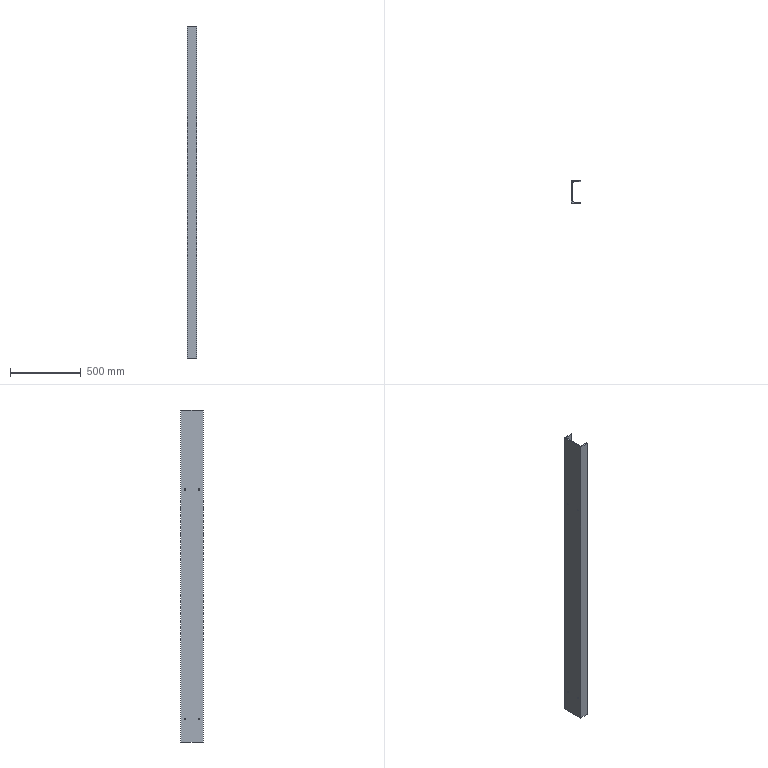Part | SolidWorks | features Extrusion 1, HoleWzd 1 | 1 solid | 18 faces | box 65 x 160 x 2340 mm | volume 4766991 mm3 | plane 10 | cylinder 8 | commonest cylinder face diameters 8.5 x8
STEP:
#1=CARTESIAN_POINT('',(8.5,30.,-1014.25));
#2=VERTEX_POINT('',#1);
#3=CARTESIAN_POINT('',(8.5,30.,-1005.75));
#4=VERTEX_POINT('',#3);
#5=CARTESIAN_POINT('',(8.5,30.,-1010.));
#6=DIRECTION('',(-1.,0.,0.));
#7=DIRECTION('',(0.,0.,1.));
#8=AXIS2_PLACEMENT_3D('',#5,#6,#7);
#9=CIRCLE('',#8,4.25);
#10=EDGE_CURVE('',#2,#4,#9,.T.);
#11=ORIENTED_EDGE('',*,*,#10,.F.);
#12=CARTESIAN_POINT('',(0.,30.,-1014.25));
#13=VERTEX_POINT('',#12);
#14=CARTESIAN_POINT('',(0.,30.,-1014.25));
#15=DIRECTION('',(-1.,0.,0.));
#16=VECTOR('',#15,1000.);
#17=LINE('',#14,#16);
#18=EDGE_CURVE('',#2,#13,#17,.T.);
#19=ORIENTED_EDGE('',*,*,#18,.T.);
#20=CARTESIAN_POINT('',(0.,30.,-1005.75));
#21=VERTEX_POINT('',#20);
#22=CARTESIAN_POINT('',(0.,30.,-1010.));
#23=DIRECTION('',(-1.,0.,0.));
#24=DIRECTION('',(0.,0.,1.));
#25=AXIS2_PLACEMENT_3D('',#22,#23,#24);
#26=CIRCLE('',#25,4.25);
#27=EDGE_CURVE('',#13,#21,#26,.T.);
#28=ORIENTED_EDGE('',*,*,#27,.T.);
#29=CARTESIAN_POINT('',(0.,30.,-1005.75));
#30=DIRECTION('',(-1.,0.,0.));
#31=VECTOR('',#30,1000.);
#32=LINE('',#29,#31);
#33=EDGE_CURVE('',#4,#21,#32,.T.);
#34=ORIENTED_EDGE('',*,*,#33,.F.);
#35=EDGE_LOOP('',(#11,#19,#28,#34));
#36=FACE_OUTER_BOUND('',#35,.T.);
#37=CARTESIAN_POINT('',(0.,30.,-1010.));
#38=DIRECTION('',(-1.,0.,0.));
#39=DIRECTION('',(0.,0.,1.));
#40=AXIS2_PLACEMENT_3D('',#37,#38,#39);
#41=CYLINDRICAL_SURFACE('',#40,4.25);
#42=ADVANCED_FACE('',(#36),#41,.F.);
#43=CARTESIAN_POINT('',(8.5,30.,605.75));
#44=VERTEX_POINT('',#43);
#45=CARTESIAN_POINT('',(8.5,30.,614.25));
#46=VERTEX_POINT('',#45);
#47=CARTESIAN_POINT('',(8.5,30.,610.));
#48=DIRECTION('',(-1.,0.,0.));
#49=DIRECTION('',(0.,0.,1.));
#50=AXIS2_PLACEMENT_3D('',#47,#48,#49);
#51=CIRCLE('',#50,4.25);
#52=EDGE_CURVE('',#44,#46,#51,.T.);
#53=ORIENTED_EDGE('',*,*,#52,.F.);
#54=CARTESIAN_POINT('',(0.,30.,605.75));
#55=VERTEX_POINT('',#54);
#56=CARTESIAN_POINT('',(0.,30.,605.75));
#57=DIRECTION('',(-1.,0.,0.));
#58=VECTOR('',#57,1000.);
#59=LINE('',#56,#58);
#60=EDGE_CURVE('',#44,#55,#59,.T.);
#61=ORIENTED_EDGE('',*,*,#60,.T.);
#62=CARTESIAN_POINT('',(0.,30.,614.25));
#63=VERTEX_POINT('',#62);
#64=CARTESIAN_POINT('',(0.,30.,610.));
#65=DIRECTION('',(-1.,0.,0.));
#66=DIRECTION('',(0.,0.,1.));
#67=AXIS2_PLACEMENT_3D('',#64,#65,#66);
#68=CIRCLE('',#67,4.25);
#69=EDGE_CURVE('',#55,#63,#68,.T.);
#70=ORIENTED_EDGE('',*,*,#69,.T.);
#71=CARTESIAN_POINT('',(0.,30.,614.25));
#72=DIRECTION('',(-1.,0.,0.));
#73=VECTOR('',#72,1000.);
#74=LINE('',#71,#73);
#75=EDGE_CURVE('',#46,#63,#74,.T.);
#76=ORIENTED_EDGE('',*,*,#75,.F.);
#77=EDGE_LOOP('',(#53,#61,#70,#76));
#78=FACE_OUTER_BOUND('',#77,.T.);
#79=CARTESIAN_POINT('',(0.,30.,610.));
#80=DIRECTION('',(-1.,0.,0.));
#81=DIRECTION('',(0.,0.,1.));
#82=AXIS2_PLACEMENT_3D('',#79,#80,#81);
#83=CYLINDRICAL_SURFACE('',#82,4.25);
#84=ADVANCED_FACE('',(#78),#83,.F.);
#85=CARTESIAN_POINT('',(8.5,130.,605.75));
#86=VERTEX_POINT('',#85);
#87=CARTESIAN_POINT('',(8.5,130.,614.25));
#88=VERTEX_POINT('',#87);
#89=CARTESIAN_POINT('',(8.5,130.,610.));
#90=DIRECTION('',(-1.,0.,0.));
#91=DIRECTION('',(0.,0.,1.));
#92=AXIS2_PLACEMENT_3D('',#89,#90,#91);
#93=CIRCLE('',#92,4.25);
#94=EDGE_CURVE('',#86,#88,#93,.T.);
#95=ORIENTED_EDGE('',*,*,#94,.F.);
#96=CARTESIAN_POINT('',(0.,130.,605.75));
#97=VERTEX_POINT('',#96);
#98=CARTESIAN_POINT('',(0.,130.,605.75));
#99=DIRECTION('',(-1.,0.,0.));
#100=VECTOR('',#99,1000.);
#101=LINE('',#98,#100);
#102=EDGE_CURVE('',#86,#97,#101,.T.);
#103=ORIENTED_EDGE('',*,*,#102,.T.);
#104=CARTESIAN_POINT('',(0.,130.,614.25));
#105=VERTEX_POINT('',#104);
#106=CARTESIAN_POINT('',(0.,130.,610.));
#107=DIRECTION('',(-1.,0.,0.));
#108=DIRECTION('',(0.,0.,1.));
#109=AXIS2_PLACEMENT_3D('',#106,#107,#108);
#110=CIRCLE('',#109,4.25);
#111=EDGE_CURVE('',#97,#105,#110,.T.);
#112=ORIENTED_EDGE('',*,*,#111,.T.);
#113=CARTESIAN_POINT('',(0.,130.,614.25));
#114=DIRECTION('',(-1.,0.,0.));
#115=VECTOR('',#114,1000.);
#116=LINE('',#113,#115);
#117=EDGE_CURVE('',#88,#105,#116,.T.);
#118=ORIENTED_EDGE('',*,*,#117,.F.);
#119=EDGE_LOOP('',(#95,#103,#112,#118));
#120=FACE_OUTER_BOUND('',#119,.T.);
#121=CARTESIAN_POINT('',(0.,130.,610.));
#122=DIRECTION('',(-1.,0.,0.));
#123=DIRECTION('',(0.,0.,1.));
#124=AXIS2_PLACEMENT_3D('',#121,#122,#123);
#125=CYLINDRICAL_SURFACE('',#124,4.25);
#126=ADVANCED_FACE('',(#120),#125,.F.);
#127=CARTESIAN_POINT('',(8.5,130.,-1014.25));
#128=VERTEX_POINT('',#127);
#129=CARTESIAN_POINT('',(8.5,130.,-1005.75));
#130=VERTEX_POINT('',#129);
#131=CARTESIAN_POINT('',(8.5,130.,-1010.));
#132=DIRECTION('',(-1.,0.,0.));
#133=DIRECTION('',(0.,0.,1.));
#134=AXIS2_PLACEMENT_3D('',#131,#132,#133);
#135=CIRCLE('',#134,4.25);
#136=EDGE_CURVE('',#128,#130,#135,.T.);
#137=ORIENTED_EDGE('',*,*,#136,.F.);
#138=CARTESIAN_POINT('',(0.,130.,-1014.25));
#139=VERTEX_POINT('',#138);
#140=CARTESIAN_POINT('',(0.,130.,-1014.25));
#141=DIRECTION('',(-1.,0.,0.));
#142=VECTOR('',#141,1000.);
#143=LINE('',#140,#142);
#144=EDGE_CURVE('',#128,#139,#143,.T.);
#145=ORIENTED_EDGE('',*,*,#144,.T.);
#146=CARTESIAN_POINT('',(0.,130.,-1005.75));
#147=VERTEX_POINT('',#146);
#148=CARTESIAN_POINT('',(0.,130.,-1010.));
#149=DIRECTION('',(-1.,0.,0.));
#150=DIRECTION('',(0.,0.,1.));
#151=AXIS2_PLACEMENT_3D('',#148,#149,#150);
#152=CIRCLE('',#151,4.25);
#153=EDGE_CURVE('',#139,#147,#152,.T.);
#154=ORIENTED_EDGE('',*,*,#153,.T.);
#155=CARTESIAN_POINT('',(0.,130.,-1005.75));
#156=DIRECTION('',(-1.,0.,0.));
#157=VECTOR('',#156,1000.);
#158=LINE('',#155,#157);
#159=EDGE_CURVE('',#130,#147,#158,.T.);
#160=ORIENTED_EDGE('',*,*,#159,.F.);
#161=EDGE_LOOP('',(#137,#145,#154,#160));
#162=FACE_OUTER_BOUND('',#161,.T.);
#163=CARTESIAN_POINT('',(0.,130.,-1010.));
#164=DIRECTION('',(-1.,0.,0.));
#165=DIRECTION('',(0.,0.,1.));
#166=AXIS2_PLACEMENT_3D('',#163,#164,#165);
#167=CYLINDRICAL_SURFACE('',#166,4.25);
#168=ADVANCED_FACE('',(#162),#167,.F.);
#169=CARTESIAN_POINT('',(0.,30.,-1010.));
#170=DIRECTION('',(-1.,0.,0.));
#171=DIRECTION('',(0.,0.,1.));
#172=AXIS2_PLACEMENT_3D('',#169,#170,#171);
#173=CIRCLE('',#172,4.25);
#174=EDGE_CURVE('',#21,#13,#173,.T.);
#175=ORIENTED_EDGE('',*,*,#174,.F.);
#176=ORIENTED_EDGE('',*,*,#27,.F.);
#177=EDGE_LOOP('',(#175,#176));
#178=FACE_BOUND('',#177,.T.);
#179=CARTESIAN_POINT('',(0.,30.,610.));
#180=DIRECTION('',(-1.,0.,0.));
#181=DIRECTION('',(0.,0.,1.));
#182=AXIS2_PLACEMENT_3D('',#179,#180,#181);
#183=CIRCLE('',#182,4.25);
#184=EDGE_CURVE('',#63,#55,#183,.T.);
#185=ORIENTED_EDGE('',*,*,#184,.F.);
#186=ORIENTED_EDGE('',*,*,#69,.F.);
#187=EDGE_LOOP('',(#185,#186));
#188=FACE_BOUND('',#187,.T.);
#189=CARTESIAN_POINT('',(0.,130.,610.));
#190=DIRECTION('',(-1.,0.,0.));
#191=DIRECTION('',(0.,0.,1.));
#192=AXIS2_PLACEMENT_3D('',#189,#190,#191);
#193=CIRCLE('',#192,4.25);
#194=EDGE_CURVE('',#105,#97,#193,.T.);
#195=ORIENTED_EDGE('',*,*,#194,.F.);
#196=ORIENTED_EDGE('',*,*,#111,.F.);
#197=EDGE_LOOP('',(#195,#196));
#198=FACE_BOUND('',#197,.T.);
#199=CARTESIAN_POINT('',(0.,130.,-1010.));
#200=DIRECTION('',(-1.,0.,0.));
#201=DIRECTION('',(0.,0.,1.));
#202=AXIS2_PLACEMENT_3D('',#199,#200,#201);
#203=CIRCLE('',#202,4.25);
#204=EDGE_CURVE('',#147,#139,#203,.T.);
#205=ORIENTED_EDGE('',*,*,#204,.F.);
#206=ORIENTED_EDGE('',*,*,#153,.F.);
#207=EDGE_LOOP('',(#205,#206));
#208=FACE_BOUND('',#207,.T.);
#209=CARTESIAN_POINT('',(0.,160.,-1170.));
#210=VERTEX_POINT('',#209);
#211=CARTESIAN_POINT('',(0.,0.,-1170.));
#212=VERTEX_POINT('',#211);
#213=CARTESIAN_POINT('',(0.,0.,-1170.));
#214=DIRECTION('',(0.,-1.,0.));
#215=VECTOR('',#214,1000.);
#216=LINE('',#213,#215);
#217=EDGE_CURVE('',#210,#212,#216,.T.);
#218=ORIENTED_EDGE('',*,*,#217,.T.);
#219=CARTESIAN_POINT('',(0.,0.,1170.));
#220=VERTEX_POINT('',#219);
#221=CARTESIAN_POINT('',(0.,0.,1170.));
#222=DIRECTION('',(0.,0.,-1.));
#223=VECTOR('',#222,1000.);
#224=LINE('',#221,#223);
#225=EDGE_CURVE('',#220,#212,#224,.T.);
#226=ORIENTED_EDGE('',*,*,#225,.F.);
#227=CARTESIAN_POINT('',(0.,160.,1170.));
#228=VERTEX_POINT('',#227);
#229=CARTESIAN_POINT('',(0.,0.,1170.));
#230=DIRECTION('',(0.,-1.,0.));
#231=VECTOR('',#230,1000.);
#232=LINE('',#229,#231);
#233=EDGE_CURVE('',#228,#220,#232,.T.);
#234=ORIENTED_EDGE('',*,*,#233,.F.);
#235=CARTESIAN_POINT('',(0.,160.,1170.));
#236=DIRECTION('',(0.,0.,-1.));
#237=VECTOR('',#236,1000.);
#238=LINE('',#235,#237);
#239=EDGE_CURVE('',#228,#210,#238,.T.);
#240=ORIENTED_EDGE('',*,*,#239,.T.);
#241=EDGE_LOOP('',(#218,#226,#234,#240));
#242=FACE_OUTER_BOUND('',#241,.T.);
#243=CARTESIAN_POINT('',(0.,0.,1170.));
#244=DIRECTION('',(1.,0.,0.));
#245=DIRECTION('',(0.,0.,-1.));
#246=AXIS2_PLACEMENT_3D('',#243,#244,#245);
#247=PLANE('',#246);
#248=ADVANCED_FACE('',(#178,#188,#198,#208,#242),#247,.F.);
#249=CARTESIAN_POINT('',(65.,0.,-1170.));
#250=VERTEX_POINT('',#249);
#251=CARTESIAN_POINT('',(0.,0.,-1170.));
#252=DIRECTION('',(1.,0.,0.));
#253=VECTOR('',#252,1000.);
#254=LINE('',#251,#253);
#255=EDGE_CURVE('',#212,#250,#254,.T.);
#256=ORIENTED_EDGE('',*,*,#255,.T.);
#257=CARTESIAN_POINT('',(65.,0.,1170.));
#258=VERTEX_POINT('',#257);
#259=CARTESIAN_POINT('',(65.,0.,1170.));
#260=DIRECTION('',(0.,0.,-1.));
#261=VECTOR('',#260,1000.);
#262=LINE('',#259,#261);
#263=EDGE_CURVE('',#258,#250,#262,.T.);
#264=ORIENTED_EDGE('',*,*,#263,.F.);
#265=CARTESIAN_POINT('',(0.,0.,1170.));
#266=DIRECTION('',(1.,0.,0.));
#267=VECTOR('',#266,1000.);
#268=LINE('',#265,#267);
#269=EDGE_CURVE('',#220,#258,#268,.T.);
#270=ORIENTED_EDGE('',*,*,#269,.F.);
#271=ORIENTED_EDGE('',*,*,#225,.T.);
#272=EDGE_LOOP('',(#256,#264,#270,#271));
#273=FACE_OUTER_BOUND('',#272,.T.);
#274=CARTESIAN_POINT('',(0.,0.,1170.));
#275=DIRECTION('',(0.,1.,0.));
#276=DIRECTION('',(0.,0.,1.));
#277=AXIS2_PLACEMENT_3D('',#274,#275,#276);
#278=PLANE('',#277);
#279=ADVANCED_FACE('',(#273),#278,.F.);
#280=CARTESIAN_POINT('',(65.,4.,-1170.));
#281=VERTEX_POINT('',#280);
#282=CARTESIAN_POINT('',(65.,0.,-1170.));
#283=DIRECTION('',(0.,1.,0.));
#284=VECTOR('',#283,1000.);
#285=LINE('',#282,#284);
#286=EDGE_CURVE('',#250,#281,#285,.T.);
#287=ORIENTED_EDGE('',*,*,#286,.T.);
#288=CARTESIAN_POINT('',(65.,4.,1170.));
#289=VERTEX_POINT('',#288);
#290=CARTESIAN_POINT('',(65.,4.,1170.));
#291=DIRECTION('',(0.,0.,-1.));
#292=VECTOR('',#291,1000.);
#293=LINE('',#290,#292);
#294=EDGE_CURVE('',#289,#281,#293,.T.);
#295=ORIENTED_EDGE('',*,*,#294,.F.);
#296=CARTESIAN_POINT('',(65.,0.,1170.));
#297=DIRECTION('',(0.,1.,0.));
#298=VECTOR('',#297,1000.);
#299=LINE('',#296,#298);
#300=EDGE_CURVE('',#258,#289,#299,.T.);
#301=ORIENTED_EDGE('',*,*,#300,.F.);
#302=ORIENTED_EDGE('',*,*,#263,.T.);
#303=EDGE_LOOP('',(#287,#295,#301,#302));
#304=FACE_OUTER_BOUND('',#303,.T.);
#305=CARTESIAN_POINT('',(65.,0.,1170.));
#306=DIRECTION('',(-1.,0.,0.));
#307=DIRECTION('',(0.,0.,1.));
#308=AXIS2_PLACEMENT_3D('',#305,#306,#307);
#309=PLANE('',#308);
#310=ADVANCED_FACE('',(#304),#309,.F.);
#311=CARTESIAN_POINT('',(8.5,8.,-1170.));
#312=VERTEX_POINT('',#311);
#313=CARTESIAN_POINT('',(65.,4.,-1170.));
#314=DIRECTION('',(-0.9975,0.07062,0.));
#315=VECTOR('',#314,1000.);
#316=LINE('',#313,#315);
#317=EDGE_CURVE('',#281,#312,#316,.T.);
#318=ORIENTED_EDGE('',*,*,#317,.T.);
#319=CARTESIAN_POINT('',(8.5,8.,1170.));
#320=VERTEX_POINT('',#319);
#321=CARTESIAN_POINT('',(8.5,8.,1170.));
#322=DIRECTION('',(0.,0.,-1.));
#323=VECTOR('',#322,1000.);
#324=LINE('',#321,#323);
#325=EDGE_CURVE('',#320,#312,#324,.T.);
#326=ORIENTED_EDGE('',*,*,#325,.F.);
#327=CARTESIAN_POINT('',(65.,4.,1170.));
#328=DIRECTION('',(-0.9975,0.07062,0.));
#329=VECTOR('',#328,1000.);
#330=LINE('',#327,#329);
#331=EDGE_CURVE('',#289,#320,#330,.T.);
#332=ORIENTED_EDGE('',*,*,#331,.F.);
#333=ORIENTED_EDGE('',*,*,#294,.T.);
#334=EDGE_LOOP('',(#318,#326,#332,#333));
#335=FACE_OUTER_BOUND('',#334,.T.);
#336=CARTESIAN_POINT('',(65.,4.,1170.));
#337=DIRECTION('',(-0.07062,-0.9975,0.));
#338=DIRECTION('',(0.9975,-0.07062,0.));
#339=AXIS2_PLACEMENT_3D('',#336,#337,#338);
#340=PLANE('',#339);
#341=ADVANCED_FACE('',(#335),#340,.F.);
#342=CARTESIAN_POINT('',(8.5,30.,-1010.));
#343=DIRECTION('',(-1.,0.,0.));
#344=DIRECTION('',(0.,0.,1.));
#345=AXIS2_PLACEMENT_3D('',#342,#343,#344);
#346=CIRCLE('',#345,4.25);
#347=EDGE_CURVE('',#4,#2,#346,.T.);
#348=ORIENTED_EDGE('',*,*,#347,.T.);
#349=ORIENTED_EDGE('',*,*,#10,.T.);
#350=EDGE_LOOP('',(#348,#349));
#351=FACE_BOUND('',#350,.T.);
#352=CARTESIAN_POINT('',(8.5,30.,610.));
#353=DIRECTION('',(-1.,0.,0.));
#354=DIRECTION('',(0.,0.,1.));
#355=AXIS2_PLACEMENT_3D('',#352,#353,#354);
#356=CIRCLE('',#355,4.25);
#357=EDGE_CURVE('',#46,#44,#356,.T.);
#358=ORIENTED_EDGE('',*,*,#357,.T.);
#359=ORIENTED_EDGE('',*,*,#52,.T.);
#360=EDGE_LOOP('',(#358,#359));
#361=FACE_BOUND('',#360,.T.);
#362=CARTESIAN_POINT('',(8.5,130.,610.));
#363=DIRECTION('',(-1.,0.,0.));
#364=DIRECTION('',(0.,0.,1.));
#365=AXIS2_PLACEMENT_3D('',#362,#363,#364);
#366=CIRCLE('',#365,4.25);
#367=EDGE_CURVE('',#88,#86,#366,.T.);
#368=ORIENTED_EDGE('',*,*,#367,.T.);
#369=ORIENTED_EDGE('',*,*,#94,.T.);
#370=EDGE_LOOP('',(#368,#369));
#371=FACE_BOUND('',#370,.T.);
#372=CARTESIAN_POINT('',(8.5,130.,-1010.));
#373=DIRECTION('',(-1.,0.,0.));
#374=DIRECTION('',(0.,0.,1.));
#375=AXIS2_PLACEMENT_3D('',#372,#373,#374);
#376=CIRCLE('',#375,4.25);
#377=EDGE_CURVE('',#130,#128,#376,.T.);
#378=ORIENTED_EDGE('',*,*,#377,.T.);
#379=ORIENTED_EDGE('',*,*,#136,.T.);
#380=EDGE_LOOP('',(#378,#379));
#381=FACE_BOUND('',#380,.T.);
#382=CARTESIAN_POINT('',(8.5,152.,-1170.));
#383=VERTEX_POINT('',#382);
#384=CARTESIAN_POINT('',(8.5,8.,-1170.));
#385=DIRECTION('',(0.,1.,0.));
#386=VECTOR('',#385,1000.);
#387=LINE('',#384,#386);
#388=EDGE_CURVE('',#312,#383,#387,.T.);
#389=ORIENTED_EDGE('',*,*,#388,.T.);
#390=CARTESIAN_POINT('',(8.5,152.,1170.));
#391=VERTEX_POINT('',#390);
#392=CARTESIAN_POINT('',(8.5,152.,1170.));
#393=DIRECTION('',(0.,0.,-1.));
#394=VECTOR('',#393,1000.);
#395=LINE('',#392,#394);
#396=EDGE_CURVE('',#391,#383,#395,.T.);
#397=ORIENTED_EDGE('',*,*,#396,.F.);
#398=CARTESIAN_POINT('',(8.5,8.,1170.));
#399=DIRECTION('',(0.,1.,0.));
#400=VECTOR('',#399,1000.);
#401=LINE('',#398,#400);
#402=EDGE_CURVE('',#320,#391,#401,.T.);
#403=ORIENTED_EDGE('',*,*,#402,.F.);
#404=ORIENTED_EDGE('',*,*,#325,.T.);
#405=EDGE_LOOP('',(#389,#397,#403,#404));
#406=FACE_OUTER_BOUND('',#405,.T.);
#407=CARTESIAN_POINT('',(8.5,8.,1170.));
#408=DIRECTION('',(-1.,0.,0.));
#409=DIRECTION('',(0.,0.,1.));
#410=AXIS2_PLACEMENT_3D('',#407,#408,#409);
#411=PLANE('',#410);
#412=ADVANCED_FACE('',(#351,#361,#371,#381,#406),#411,.F.);
#413=CARTESIAN_POINT('',(65.,156.,-1170.));
#414=VERTEX_POINT('',#413);
#415=CARTESIAN_POINT('',(65.,156.,-1170.));
#416=DIRECTION('',(0.9975,0.07062,0.));
#417=VECTOR('',#416,1000.);
#418=LINE('',#415,#417);
#419=EDGE_CURVE('',#383,#414,#418,.T.);
#420=ORIENTED_EDGE('',*,*,#419,.T.);
#421=CARTESIAN_POINT('',(65.,156.,1170.));
#422=VERTEX_POINT('',#421);
#423=CARTESIAN_POINT('',(65.,156.,1170.));
#424=DIRECTION('',(0.,0.,-1.));
#425=VECTOR('',#424,1000.);
#426=LINE('',#423,#425);
#427=EDGE_CURVE('',#422,#414,#426,.T.);
#428=ORIENTED_EDGE('',*,*,#427,.F.);
#429=CARTESIAN_POINT('',(65.,156.,1170.));
#430=DIRECTION('',(0.9975,0.07062,0.));
#431=VECTOR('',#430,1000.);
#432=LINE('',#429,#431);
#433=EDGE_CURVE('',#391,#422,#432,.T.);
#434=ORIENTED_EDGE('',*,*,#433,.F.);
#435=ORIENTED_EDGE('',*,*,#396,.T.);
#436=EDGE_LOOP('',(#420,#428,#434,#435));
#437=FACE_OUTER_BOUND('',#436,.T.);
#438=CARTESIAN_POINT('',(65.,156.,1170.));
#439=DIRECTION('',(-0.07062,0.9975,0.));
#440=DIRECTION('',(-0.9975,-0.07062,0.));
#441=AXIS2_PLACEMENT_3D('',#438,#439,#440);
#442=PLANE('',#441);
#443=ADVANCED_FACE('',(#437),#442,.F.);
#444=CARTESIAN_POINT('',(65.,160.,-1170.));
#445=VERTEX_POINT('',#444);
#446=CARTESIAN_POINT('',(65.,160.,-1170.));
#447=DIRECTION('',(0.,1.,0.));
#448=VECTOR('',#447,1000.);
#449=LINE('',#446,#448);
#450=EDGE_CURVE('',#414,#445,#449,.T.);
#451=ORIENTED_EDGE('',*,*,#450,.T.);
#452=CARTESIAN_POINT('',(65.,160.,1170.));
#453=VERTEX_POINT('',#452);
#454=CARTESIAN_POINT('',(65.,160.,1170.));
#455=DIRECTION('',(0.,0.,-1.));
#456=VECTOR('',#455,1000.);
#457=LINE('',#454,#456);
#458=EDGE_CURVE('',#453,#445,#457,.T.);
#459=ORIENTED_EDGE('',*,*,#458,.F.);
#460=CARTESIAN_POINT('',(65.,160.,1170.));
#461=DIRECTION('',(0.,1.,0.));
#462=VECTOR('',#461,1000.);
#463=LINE('',#460,#462);
#464=EDGE_CURVE('',#422,#453,#463,.T.);
#465=ORIENTED_EDGE('',*,*,#464,.F.);
#466=ORIENTED_EDGE('',*,*,#427,.T.);
#467=EDGE_LOOP('',(#451,#459,#465,#466));
#468=FACE_OUTER_BOUND('',#467,.T.);
#469=CARTESIAN_POINT('',(65.,160.,1170.));
#470=DIRECTION('',(-1.,0.,0.));
#471=DIRECTION('',(0.,0.,1.));
#472=AXIS2_PLACEMENT_3D('',#469,#470,#471);
#473=PLANE('',#472);
#474=ADVANCED_FACE('',(#468),#473,.F.);
#475=CARTESIAN_POINT('',(0.,160.,-1170.));
#476=DIRECTION('',(-1.,0.,0.));
#477=VECTOR('',#476,1000.);
#478=LINE('',#475,#477);
#479=EDGE_CURVE('',#445,#210,#478,.T.);
#480=ORIENTED_EDGE('',*,*,#479,.T.);
#481=ORIENTED_EDGE('',*,*,#239,.F.);
#482=CARTESIAN_POINT('',(0.,160.,1170.));
#483=DIRECTION('',(-1.,0.,0.));
#484=VECTOR('',#483,1000.);
#485=LINE('',#482,#484);
#486=EDGE_CURVE('',#453,#228,#485,.T.);
#487=ORIENTED_EDGE('',*,*,#486,.F.);
#488=ORIENTED_EDGE('',*,*,#458,.T.);
#489=EDGE_LOOP('',(#480,#481,#487,#488));
#490=FACE_OUTER_BOUND('',#489,.T.);
#491=CARTESIAN_POINT('',(0.,160.,1170.));
#492=DIRECTION('',(0.,-1.,0.));
#493=DIRECTION('',(1.,0.,0.));
#494=AXIS2_PLACEMENT_3D('',#491,#492,#493);
#495=PLANE('',#494);
#496=ADVANCED_FACE('',(#490),#495,.F.);
#497=ORIENTED_EDGE('',*,*,#233,.T.);
#498=ORIENTED_EDGE('',*,*,#269,.T.);
#499=ORIENTED_EDGE('',*,*,#300,.T.);
#500=ORIENTED_EDGE('',*,*,#331,.T.);
#501=ORIENTED_EDGE('',*,*,#402,.T.);
#502=ORIENTED_EDGE('',*,*,#433,.T.);
#503=ORIENTED_EDGE('',*,*,#464,.T.);
#504=ORIENTED_EDGE('',*,*,#486,.T.);
#505=EDGE_LOOP('',(#497,#498,#499,#500,#501,#502,#503,#504));
#506=FACE_OUTER_BOUND('',#505,.T.);
#507=CARTESIAN_POINT('',(0.,0.,1170.));
#508=DIRECTION('',(0.,0.,-1.));
#509=DIRECTION('',(-1.,0.,0.));
#510=AXIS2_PLACEMENT_3D('',#507,#508,#509);
#511=PLANE('',#510);
#512=ADVANCED_FACE('',(#506),#511,.F.);
#513=ORIENTED_EDGE('',*,*,#217,.F.);
#514=ORIENTED_EDGE('',*,*,#479,.F.);
#515=ORIENTED_EDGE('',*,*,#450,.F.);
#516=ORIENTED_EDGE('',*,*,#419,.F.);
#517=ORIENTED_EDGE('',*,*,#388,.F.);
#518=ORIENTED_EDGE('',*,*,#317,.F.);
#519=ORIENTED_EDGE('',*,*,#286,.F.);
#520=ORIENTED_EDGE('',*,*,#255,.F.);
#521=EDGE_LOOP('',(#513,#514,#515,#516,#517,#518,#519,#520));
#522=FACE_OUTER_BOUND('',#521,.T.);
#523=CARTESIAN_POINT('',(0.,0.,-1170.));
#524=DIRECTION('',(0.,0.,-1.));
#525=DIRECTION('',(-1.,0.,0.));
#526=AXIS2_PLACEMENT_3D('',#523,#524,#525);
#527=PLANE('',#526);
#528=ADVANCED_FACE('',(#522),#527,.T.);
#529=ORIENTED_EDGE('',*,*,#144,.F.);
#530=ORIENTED_EDGE('',*,*,#377,.F.);
#531=ORIENTED_EDGE('',*,*,#159,.T.);
#532=ORIENTED_EDGE('',*,*,#204,.T.);
#533=EDGE_LOOP('',(#529,#530,#531,#532));
#534=FACE_OUTER_BOUND('',#533,.T.);
#535=CARTESIAN_POINT('',(0.,130.,-1010.));
#536=DIRECTION('',(-1.,0.,0.));
#537=DIRECTION('',(0.,0.,1.));
#538=AXIS2_PLACEMENT_3D('',#535,#536,#537);
#539=CYLINDRICAL_SURFACE('',#538,4.25);
#540=ADVANCED_FACE('',(#534),#539,.F.);
#541=ORIENTED_EDGE('',*,*,#102,.F.);
#542=ORIENTED_EDGE('',*,*,#367,.F.);
#543=ORIENTED_EDGE('',*,*,#117,.T.);
#544=ORIENTED_EDGE('',*,*,#194,.T.);
#545=EDGE_LOOP('',(#541,#542,#543,#544));
#546=FACE_OUTER_BOUND('',#545,.T.);
#547=CARTESIAN_POINT('',(0.,130.,610.));
#548=DIRECTION('',(-1.,0.,0.));
#549=DIRECTION('',(0.,0.,1.));
#550=AXIS2_PLACEMENT_3D('',#547,#548,#549);
#551=CYLINDRICAL_SURFACE('',#550,4.25);
#552=ADVANCED_FACE('',(#546),#551,.F.);
#553=ORIENTED_EDGE('',*,*,#60,.F.);
#554=ORIENTED_EDGE('',*,*,#357,.F.);
#555=ORIENTED_EDGE('',*,*,#75,.T.);
#556=ORIENTED_EDGE('',*,*,#184,.T.);
#557=EDGE_LOOP('',(#553,#554,#555,#556));
#558=FACE_OUTER_BOUND('',#557,.T.);
#559=CARTESIAN_POINT('',(0.,30.,610.));
#560=DIRECTION('',(-1.,0.,0.));
#561=DIRECTION('',(0.,0.,1.));
#562=AXIS2_PLACEMENT_3D('',#559,#560,#561);
#563=CYLINDRICAL_SURFACE('',#562,4.25);
#564=ADVANCED_FACE('',(#558),#563,.F.);
#565=ORIENTED_EDGE('',*,*,#18,.F.);
#566=ORIENTED_EDGE('',*,*,#347,.F.);
#567=ORIENTED_EDGE('',*,*,#33,.T.);
#568=ORIENTED_EDGE('',*,*,#174,.T.);
#569=EDGE_LOOP('',(#565,#566,#567,#568));
#570=FACE_OUTER_BOUND('',#569,.T.);
#571=CARTESIAN_POINT('',(0.,30.,-1010.));
#572=DIRECTION('',(-1.,0.,0.));
#573=DIRECTION('',(0.,0.,1.));
#574=AXIS2_PLACEMENT_3D('',#571,#572,#573);
#575=CYLINDRICAL_SURFACE('',#574,4.25);
#576=ADVANCED_FACE('',(#570),#575,.F.);
#577=CLOSED_SHELL('',(#42,#84,#126,#168,#248,#279,#310,#341,#412,#443,#474,#496,#512,#528,#540,#552,#564,#576));
#578=MANIFOLD_SOLID_BREP('',#577);
#579=CARTESIAN_POINT('',(0.,0.,0.));
#580=DIRECTION('',(0.,0.,1.));
#581=DIRECTION('',(1.,0.,0.));
#582=AXIS2_PLACEMENT_3D('',#579,#580,#581);
#583=(LENGTH_UNIT()NAMED_UNIT(*)SI_UNIT(.MILLI.,.METRE.));
#584=UNCERTAINTY_MEASURE_WITH_UNIT(LENGTH_MEASURE(0.00001),#583,'','');
#585=(NAMED_UNIT(*)PLANE_ANGLE_UNIT()SI_UNIT($,.RADIAN.));
#586=(NAMED_UNIT(*)SI_UNIT($,.STERADIAN.)SOLID_ANGLE_UNIT());
#587=(GEOMETRIC_REPRESENTATION_CONTEXT(3)GLOBAL_UNCERTAINTY_ASSIGNED_CONTEXT((#584))GLOBAL_UNIT_ASSIGNED_CONTEXT((#583,#585,#586))REPRESENTATION_CONTEXT('',''));
#588=ADVANCED_BREP_SHAPE_REPRESENTATION('',(#578,#582),#587);